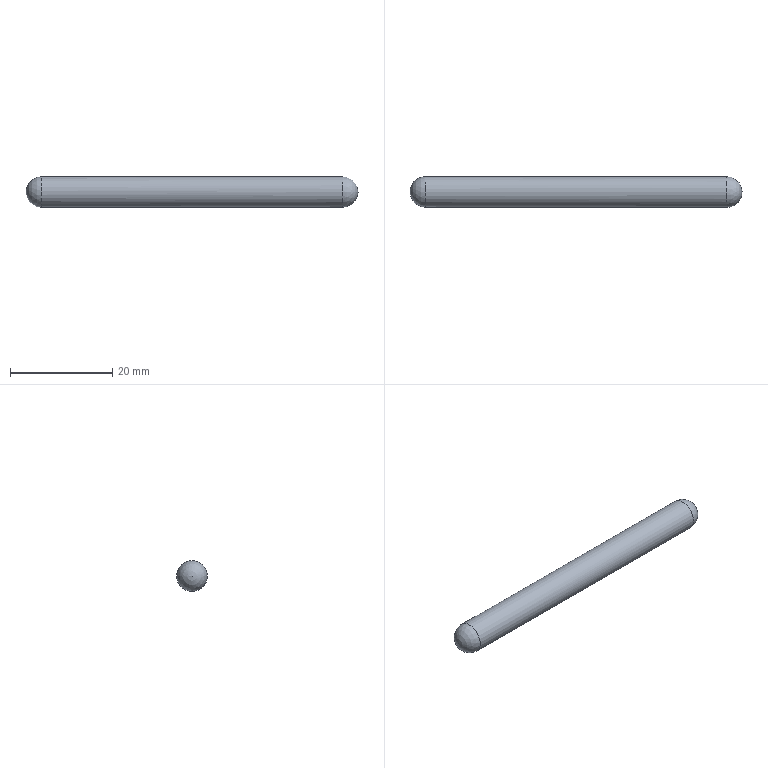Part | NX | 1 solid | 3 faces | box 65 x 6 x 6 mm | volume 1781 mm3 | sphere 2 | cylinder 1 | commonest cylinder face diameters 6 x1
STEP:
#1=CARTESIAN_POINT('',(3.,0.,3.));
#2=VERTEX_POINT('',#1);
#3=CARTESIAN_POINT('',(3.,0.,0.));
#4=DIRECTION('',(-1.,0.,0.));
#5=DIRECTION('',(0.,0.,1.));
#6=AXIS2_PLACEMENT_3D('',#3,#4,#5);
#7=CIRCLE('',#6,3.);
#8=EDGE_CURVE('',#2,#2,#7,.T.);
#9=ORIENTED_EDGE('',*,*,#8,.T.);
#10=EDGE_LOOP('',(#9));
#11=FACE_BOUND('',#10,.T.);
#12=CARTESIAN_POINT('',(3.,0.,0.));
#13=DIRECTION('',(-1.,0.,0.));
#14=DIRECTION('',(0.,1.,0.));
#15=AXIS2_PLACEMENT_3D('',#12,#13,#14);
#16=SPHERICAL_SURFACE('',#15,3.);
#17=ADVANCED_FACE('',(#11),#16,.T.);
#18=ORIENTED_EDGE('',*,*,#8,.F.);
#19=EDGE_LOOP('',(#18));
#20=FACE_BOUND('',#19,.T.);
#21=CARTESIAN_POINT('',(62.,0.,3.));
#22=VERTEX_POINT('',#21);
#23=CARTESIAN_POINT('',(62.,0.,0.));
#24=DIRECTION('',(-1.,0.,0.));
#25=DIRECTION('',(0.,0.,1.));
#26=AXIS2_PLACEMENT_3D('',#23,#24,#25);
#27=CIRCLE('',#26,3.);
#28=EDGE_CURVE('',#22,#22,#27,.T.);
#29=ORIENTED_EDGE('',*,*,#28,.T.);
#30=EDGE_LOOP('',(#29));
#31=FACE_BOUND('',#30,.T.);
#32=CARTESIAN_POINT('',(65.,0.,0.));
#33=DIRECTION('',(-1.,0.,0.));
#34=DIRECTION('',(0.,0.,1.));
#35=AXIS2_PLACEMENT_3D('',#32,#33,#34);
#36=CYLINDRICAL_SURFACE('',#35,3.);
#37=ADVANCED_FACE('',(#20,#31),#36,.T.);
#38=ORIENTED_EDGE('',*,*,#28,.F.);
#39=EDGE_LOOP('',(#38));
#40=FACE_BOUND('',#39,.T.);
#41=CARTESIAN_POINT('',(62.,0.,0.));
#42=DIRECTION('',(-1.,0.,0.));
#43=DIRECTION('',(0.,-1.,0.));
#44=AXIS2_PLACEMENT_3D('',#41,#42,#43);
#45=SPHERICAL_SURFACE('',#44,3.);
#46=ADVANCED_FACE('',(#40),#45,.T.);
#47=CLOSED_SHELL('',(#17,#37,#46));
#48=MANIFOLD_SOLID_BREP('',#47);
#49=(LENGTH_UNIT()NAMED_UNIT(*)SI_UNIT(.MILLI.,.METRE.));
#50=UNCERTAINTY_MEASURE_WITH_UNIT(LENGTH_MEASURE(0.00001),#49,'','');
#51=(NAMED_UNIT(*)PLANE_ANGLE_UNIT()SI_UNIT($,.RADIAN.));
#52=(NAMED_UNIT(*)SI_UNIT($,.STERADIAN.)SOLID_ANGLE_UNIT());
#53=(GEOMETRIC_REPRESENTATION_CONTEXT(3)GLOBAL_UNCERTAINTY_ASSIGNED_CONTEXT((#50))GLOBAL_UNIT_ASSIGNED_CONTEXT((#49,#51,#52))REPRESENTATION_CONTEXT('',''));
#54=ADVANCED_BREP_SHAPE_REPRESENTATION('',(#48),#53);